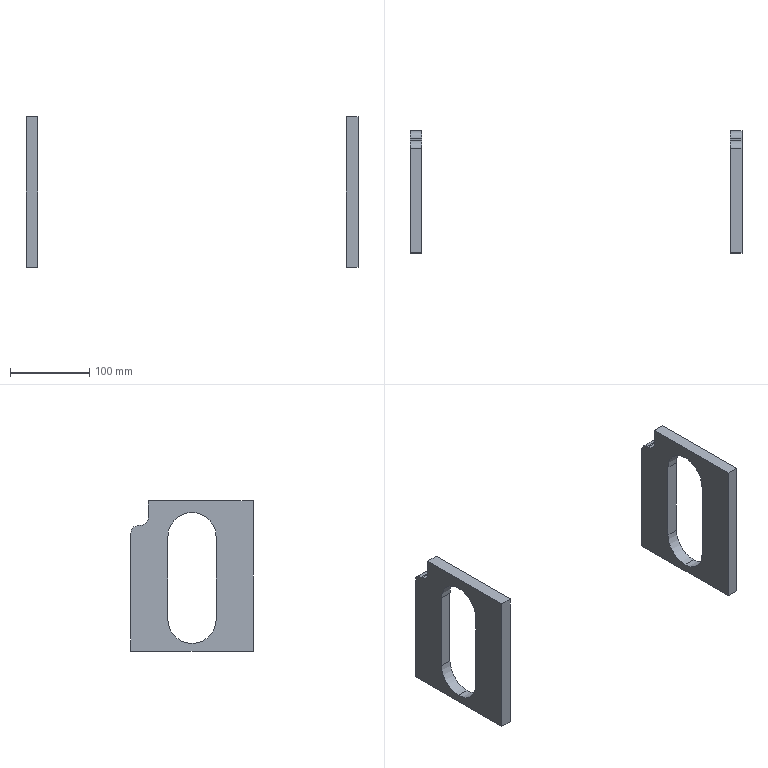Part | STEP file | Part 14^超升波生产线-2 | 2 solids | 30 faces | box 420 x 154.525 x 190 mm | volume 580946 mm3 | plane 20 | cylinder 10 | commonest cylinder face diameters 61.047 x6 20 x4
STEP:
#1=CARTESIAN_POINT('',(195.,0.,9.642));
#2=VERTEX_POINT('',#1);
#3=CARTESIAN_POINT('',(195.,30.523,40.165));
#4=VERTEX_POINT('',#3);
#5=CARTESIAN_POINT('',(195.,0.,40.165));
#6=DIRECTION('',(1.,0.,0.));
#7=DIRECTION('',(0.,1.,0.));
#8=AXIS2_PLACEMENT_3D('',#5,#6,#7);
#9=CIRCLE('',#8,30.523);
#10=EDGE_CURVE('',#2,#4,#9,.T.);
#11=ORIENTED_EDGE('',*,*,#10,.F.);
#12=CARTESIAN_POINT('',(210.,0.,9.642));
#13=VERTEX_POINT('',#12);
#14=CARTESIAN_POINT('',(-210.,0.,9.642));
#15=DIRECTION('',(1.,0.,0.));
#16=VECTOR('',#15,1000.);
#17=LINE('',#14,#16);
#18=EDGE_CURVE('',#2,#13,#17,.T.);
#19=ORIENTED_EDGE('',*,*,#18,.T.);
#20=CARTESIAN_POINT('',(210.,30.523,40.165));
#21=VERTEX_POINT('',#20);
#22=CARTESIAN_POINT('',(210.,0.,40.165));
#23=DIRECTION('',(1.,0.,0.));
#24=DIRECTION('',(0.,0.,-1.));
#25=AXIS2_PLACEMENT_3D('',#22,#23,#24);
#26=CIRCLE('',#25,30.523);
#27=EDGE_CURVE('',#13,#21,#26,.T.);
#28=ORIENTED_EDGE('',*,*,#27,.T.);
#29=CARTESIAN_POINT('',(-210.,30.523,40.165));
#30=DIRECTION('',(1.,0.,0.));
#31=VECTOR('',#30,1000.);
#32=LINE('',#29,#31);
#33=EDGE_CURVE('',#4,#21,#32,.T.);
#34=ORIENTED_EDGE('',*,*,#33,.F.);
#35=EDGE_LOOP('',(#11,#19,#28,#34));
#36=FACE_OUTER_BOUND('',#35,.T.);
#37=CARTESIAN_POINT('',(-210.,0.,40.165));
#38=DIRECTION('',(1.,0.,0.));
#39=DIRECTION('',(0.,0.,-1.));
#40=AXIS2_PLACEMENT_3D('',#37,#38,#39);
#41=CYLINDRICAL_SURFACE('',#40,30.523);
#42=ADVANCED_FACE('',(#36),#41,.F.);
#43=CARTESIAN_POINT('',(210.,-30.523,144.796));
#44=VERTEX_POINT('',#43);
#45=CARTESIAN_POINT('',(210.,-30.523,40.165));
#46=VERTEX_POINT('',#45);
#47=CARTESIAN_POINT('',(210.,-30.523,144.796));
#48=DIRECTION('',(0.,0.,-1.));
#49=VECTOR('',#48,1000.);
#50=LINE('',#47,#49);
#51=EDGE_CURVE('',#44,#46,#50,.T.);
#52=ORIENTED_EDGE('',*,*,#51,.F.);
#53=CARTESIAN_POINT('',(210.,30.523,144.796));
#54=VERTEX_POINT('',#53);
#55=CARTESIAN_POINT('',(210.,0.,144.796));
#56=DIRECTION('',(1.,0.,0.));
#57=DIRECTION('',(0.,0.,-1.));
#58=AXIS2_PLACEMENT_3D('',#55,#56,#57);
#59=CIRCLE('',#58,30.523);
#60=EDGE_CURVE('',#54,#44,#59,.T.);
#61=ORIENTED_EDGE('',*,*,#60,.F.);
#62=CARTESIAN_POINT('',(210.,30.523,144.796));
#63=DIRECTION('',(0.,0.,1.));
#64=VECTOR('',#63,1000.);
#65=LINE('',#62,#64);
#66=EDGE_CURVE('',#21,#54,#65,.T.);
#67=ORIENTED_EDGE('',*,*,#66,.F.);
#68=ORIENTED_EDGE('',*,*,#27,.F.);
#69=CARTESIAN_POINT('',(210.,0.,40.165));
#70=DIRECTION('',(1.,0.,0.));
#71=DIRECTION('',(0.,0.,-1.));
#72=AXIS2_PLACEMENT_3D('',#69,#70,#71);
#73=CIRCLE('',#72,30.523);
#74=EDGE_CURVE('',#46,#13,#73,.T.);
#75=ORIENTED_EDGE('',*,*,#74,.F.);
#76=EDGE_LOOP('',(#52,#61,#67,#68,#75));
#77=FACE_BOUND('',#76,.T.);
#78=CARTESIAN_POINT('',(210.,77.262,149.237));
#79=VERTEX_POINT('',#78);
#80=CARTESIAN_POINT('',(210.,77.262,0.));
#81=VERTEX_POINT('',#80);
#82=CARTESIAN_POINT('',(210.,77.262,190.));
#83=DIRECTION('',(0.,0.,-1.));
#84=VECTOR('',#83,1000.);
#85=LINE('',#82,#84);
#86=EDGE_CURVE('',#79,#81,#85,.T.);
#87=ORIENTED_EDGE('',*,*,#86,.F.);
#88=CARTESIAN_POINT('',(210.,67.262,159.237));
#89=VERTEX_POINT('',#88);
#90=CARTESIAN_POINT('',(210.,67.262,149.237));
#91=DIRECTION('',(1.,0.,0.));
#92=DIRECTION('',(0.,0.,1.));
#93=AXIS2_PLACEMENT_3D('',#90,#91,#92);
#94=CIRCLE('',#93,10.);
#95=EDGE_CURVE('',#79,#89,#94,.T.);
#96=ORIENTED_EDGE('',*,*,#95,.T.);
#97=CARTESIAN_POINT('',(210.,65.138,159.237));
#98=VERTEX_POINT('',#97);
#99=CARTESIAN_POINT('',(210.,79.238,159.237));
#100=DIRECTION('',(0.,-1.,0.));
#101=VECTOR('',#100,1000.);
#102=LINE('',#99,#101);
#103=EDGE_CURVE('',#89,#98,#102,.T.);
#104=ORIENTED_EDGE('',*,*,#103,.T.);
#105=CARTESIAN_POINT('',(210.,55.138,169.237));
#106=VERTEX_POINT('',#105);
#107=CARTESIAN_POINT('',(210.,65.138,169.237));
#108=DIRECTION('',(-1.,0.,0.));
#109=DIRECTION('',(0.,0.,1.));
#110=AXIS2_PLACEMENT_3D('',#107,#108,#109);
#111=CIRCLE('',#110,10.);
#112=EDGE_CURVE('',#98,#106,#111,.T.);
#113=ORIENTED_EDGE('',*,*,#112,.T.);
#114=CARTESIAN_POINT('',(210.,55.138,190.));
#115=VERTEX_POINT('',#114);
#116=CARTESIAN_POINT('',(210.,55.138,192.637));
#117=DIRECTION('',(0.,0.,1.));
#118=VECTOR('',#117,1000.);
#119=LINE('',#116,#118);
#120=EDGE_CURVE('',#106,#115,#119,.T.);
#121=ORIENTED_EDGE('',*,*,#120,.T.);
#122=CARTESIAN_POINT('',(210.,-77.262,190.));
#123=VERTEX_POINT('',#122);
#124=CARTESIAN_POINT('',(210.,77.262,190.));
#125=DIRECTION('',(0.,1.,0.));
#126=VECTOR('',#125,1000.);
#127=LINE('',#124,#126);
#128=EDGE_CURVE('',#123,#115,#127,.T.);
#129=ORIENTED_EDGE('',*,*,#128,.F.);
#130=CARTESIAN_POINT('',(210.,-77.262,0.));
#131=VERTEX_POINT('',#130);
#132=CARTESIAN_POINT('',(210.,-77.262,190.));
#133=DIRECTION('',(0.,0.,-1.));
#134=VECTOR('',#133,1000.);
#135=LINE('',#132,#134);
#136=EDGE_CURVE('',#123,#131,#135,.T.);
#137=ORIENTED_EDGE('',*,*,#136,.T.);
#138=CARTESIAN_POINT('',(210.,77.262,0.));
#139=DIRECTION('',(0.,1.,0.));
#140=VECTOR('',#139,1000.);
#141=LINE('',#138,#140);
#142=EDGE_CURVE('',#131,#81,#141,.T.);
#143=ORIENTED_EDGE('',*,*,#142,.T.);
#144=EDGE_LOOP('',(#87,#96,#104,#113,#121,#129,#137,#143));
#145=FACE_OUTER_BOUND('',#144,.T.);
#146=CARTESIAN_POINT('',(210.,77.262,190.));
#147=DIRECTION('',(-1.,0.,0.));
#148=DIRECTION('',(0.,0.,1.));
#149=AXIS2_PLACEMENT_3D('',#146,#147,#148);
#150=PLANE('',#149);
#151=ADVANCED_FACE('',(#77,#145),#150,.F.);
#152=CARTESIAN_POINT('',(195.,77.262,149.237));
#153=VERTEX_POINT('',#152);
#154=CARTESIAN_POINT('',(195.,77.262,0.));
#155=VERTEX_POINT('',#154);
#156=CARTESIAN_POINT('',(195.,77.262,190.));
#157=DIRECTION('',(0.,0.,-1.));
#158=VECTOR('',#157,1000.);
#159=LINE('',#156,#158);
#160=EDGE_CURVE('',#153,#155,#159,.T.);
#161=ORIENTED_EDGE('',*,*,#160,.F.);
#162=CARTESIAN_POINT('',(210.,77.262,149.237));
#163=DIRECTION('',(1.,0.,0.));
#164=VECTOR('',#163,1000.);
#165=LINE('',#162,#164);
#166=EDGE_CURVE('',#153,#79,#165,.T.);
#167=ORIENTED_EDGE('',*,*,#166,.T.);
#168=ORIENTED_EDGE('',*,*,#86,.T.);
#169=CARTESIAN_POINT('',(210.,77.262,0.));
#170=DIRECTION('',(-1.,0.,0.));
#171=VECTOR('',#170,1000.);
#172=LINE('',#169,#171);
#173=EDGE_CURVE('',#81,#155,#172,.T.);
#174=ORIENTED_EDGE('',*,*,#173,.T.);
#175=EDGE_LOOP('',(#161,#167,#168,#174));
#176=FACE_OUTER_BOUND('',#175,.T.);
#177=CARTESIAN_POINT('',(210.,77.262,190.));
#178=DIRECTION('',(0.,-1.,0.));
#179=DIRECTION('',(0.,0.,-1.));
#180=AXIS2_PLACEMENT_3D('',#177,#178,#179);
#181=PLANE('',#180);
#182=ADVANCED_FACE('',(#176),#181,.F.);
#183=CARTESIAN_POINT('',(195.,30.523,144.796));
#184=VERTEX_POINT('',#183);
#185=CARTESIAN_POINT('',(195.,30.523,190.));
#186=DIRECTION('',(0.,0.,1.));
#187=VECTOR('',#186,1000.);
#188=LINE('',#185,#187);
#189=EDGE_CURVE('',#4,#184,#188,.T.);
#190=ORIENTED_EDGE('',*,*,#189,.T.);
#191=CARTESIAN_POINT('',(195.,-30.523,144.796));
#192=VERTEX_POINT('',#191);
#193=CARTESIAN_POINT('',(195.,0.,144.796));
#194=DIRECTION('',(1.,0.,0.));
#195=DIRECTION('',(0.,1.,0.));
#196=AXIS2_PLACEMENT_3D('',#193,#194,#195);
#197=CIRCLE('',#196,30.523);
#198=EDGE_CURVE('',#184,#192,#197,.T.);
#199=ORIENTED_EDGE('',*,*,#198,.T.);
#200=CARTESIAN_POINT('',(195.,-30.523,40.165));
#201=VERTEX_POINT('',#200);
#202=CARTESIAN_POINT('',(195.,-30.523,190.));
#203=DIRECTION('',(0.,0.,-1.));
#204=VECTOR('',#203,1000.);
#205=LINE('',#202,#204);
#206=EDGE_CURVE('',#192,#201,#205,.T.);
#207=ORIENTED_EDGE('',*,*,#206,.T.);
#208=CARTESIAN_POINT('',(195.,0.,40.165));
#209=DIRECTION('',(1.,0.,0.));
#210=DIRECTION('',(0.,1.,0.));
#211=AXIS2_PLACEMENT_3D('',#208,#209,#210);
#212=CIRCLE('',#211,30.523);
#213=EDGE_CURVE('',#201,#2,#212,.T.);
#214=ORIENTED_EDGE('',*,*,#213,.T.);
#215=ORIENTED_EDGE('',*,*,#10,.T.);
#216=EDGE_LOOP('',(#190,#199,#207,#214,#215));
#217=FACE_BOUND('',#216,.T.);
#218=CARTESIAN_POINT('',(195.,65.138,159.237));
#219=VERTEX_POINT('',#218);
#220=CARTESIAN_POINT('',(195.,67.262,159.237));
#221=VERTEX_POINT('',#220);
#222=CARTESIAN_POINT('',(195.,77.262,159.237));
#223=DIRECTION('',(0.,1.,0.));
#224=VECTOR('',#223,1000.);
#225=LINE('',#222,#224);
#226=EDGE_CURVE('',#219,#221,#225,.T.);
#227=ORIENTED_EDGE('',*,*,#226,.T.);
#228=CARTESIAN_POINT('',(195.,67.262,149.237));
#229=DIRECTION('',(-1.,0.,0.));
#230=DIRECTION('',(0.,1.,0.));
#231=AXIS2_PLACEMENT_3D('',#228,#229,#230);
#232=CIRCLE('',#231,10.);
#233=EDGE_CURVE('',#221,#153,#232,.T.);
#234=ORIENTED_EDGE('',*,*,#233,.T.);
#235=ORIENTED_EDGE('',*,*,#160,.T.);
#236=CARTESIAN_POINT('',(195.,-77.262,0.));
#237=VERTEX_POINT('',#236);
#238=CARTESIAN_POINT('',(195.,77.262,0.));
#239=DIRECTION('',(0.,-1.,0.));
#240=VECTOR('',#239,1000.);
#241=LINE('',#238,#240);
#242=EDGE_CURVE('',#155,#237,#241,.T.);
#243=ORIENTED_EDGE('',*,*,#242,.T.);
#244=CARTESIAN_POINT('',(195.,-77.262,190.));
#245=VERTEX_POINT('',#244);
#246=CARTESIAN_POINT('',(195.,-77.262,190.));
#247=DIRECTION('',(0.,0.,-1.));
#248=VECTOR('',#247,1000.);
#249=LINE('',#246,#248);
#250=EDGE_CURVE('',#245,#237,#249,.T.);
#251=ORIENTED_EDGE('',*,*,#250,.F.);
#252=CARTESIAN_POINT('',(195.,55.138,190.));
#253=VERTEX_POINT('',#252);
#254=CARTESIAN_POINT('',(195.,77.262,190.));
#255=DIRECTION('',(0.,-1.,0.));
#256=VECTOR('',#255,1000.);
#257=LINE('',#254,#256);
#258=EDGE_CURVE('',#253,#245,#257,.T.);
#259=ORIENTED_EDGE('',*,*,#258,.F.);
#260=CARTESIAN_POINT('',(195.,55.138,169.237));
#261=VERTEX_POINT('',#260);
#262=CARTESIAN_POINT('',(195.,55.138,190.));
#263=DIRECTION('',(0.,0.,-1.));
#264=VECTOR('',#263,1000.);
#265=LINE('',#262,#264);
#266=EDGE_CURVE('',#253,#261,#265,.T.);
#267=ORIENTED_EDGE('',*,*,#266,.T.);
#268=CARTESIAN_POINT('',(195.,65.138,169.237));
#269=DIRECTION('',(1.,0.,0.));
#270=DIRECTION('',(0.,1.,0.));
#271=AXIS2_PLACEMENT_3D('',#268,#269,#270);
#272=CIRCLE('',#271,10.);
#273=EDGE_CURVE('',#261,#219,#272,.T.);
#274=ORIENTED_EDGE('',*,*,#273,.T.);
#275=EDGE_LOOP('',(#227,#234,#235,#243,#251,#259,#267,#274));
#276=FACE_OUTER_BOUND('',#275,.T.);
#277=CARTESIAN_POINT('',(195.,77.262,190.));
#278=DIRECTION('',(1.,0.,0.));
#279=DIRECTION('',(0.,1.,0.));
#280=AXIS2_PLACEMENT_3D('',#277,#278,#279);
#281=PLANE('',#280);
#282=ADVANCED_FACE('',(#217,#276),#281,.F.);
#283=CARTESIAN_POINT('',(210.,-77.262,0.));
#284=DIRECTION('',(1.,0.,0.));
#285=VECTOR('',#284,1000.);
#286=LINE('',#283,#285);
#287=EDGE_CURVE('',#237,#131,#286,.T.);
#288=ORIENTED_EDGE('',*,*,#287,.T.);
#289=ORIENTED_EDGE('',*,*,#136,.F.);
#290=CARTESIAN_POINT('',(210.,-77.262,190.));
#291=DIRECTION('',(1.,0.,0.));
#292=VECTOR('',#291,1000.);
#293=LINE('',#290,#292);
#294=EDGE_CURVE('',#245,#123,#293,.T.);
#295=ORIENTED_EDGE('',*,*,#294,.F.);
#296=ORIENTED_EDGE('',*,*,#250,.T.);
#297=EDGE_LOOP('',(#288,#289,#295,#296));
#298=FACE_OUTER_BOUND('',#297,.T.);
#299=CARTESIAN_POINT('',(210.,-77.262,190.));
#300=DIRECTION('',(0.,1.,0.));
#301=DIRECTION('',(0.,0.,1.));
#302=AXIS2_PLACEMENT_3D('',#299,#300,#301);
#303=PLANE('',#302);
#304=ADVANCED_FACE('',(#298),#303,.F.);
#305=ORIENTED_EDGE('',*,*,#128,.T.);
#306=CARTESIAN_POINT('',(210.,55.138,190.));
#307=DIRECTION('',(-1.,0.,0.));
#308=VECTOR('',#307,1000.);
#309=LINE('',#306,#308);
#310=EDGE_CURVE('',#115,#253,#309,.T.);
#311=ORIENTED_EDGE('',*,*,#310,.T.);
#312=ORIENTED_EDGE('',*,*,#258,.T.);
#313=ORIENTED_EDGE('',*,*,#294,.T.);
#314=EDGE_LOOP('',(#305,#311,#312,#313));
#315=FACE_OUTER_BOUND('',#314,.T.);
#316=CARTESIAN_POINT('',(210.,-77.262,190.));
#317=DIRECTION('',(0.,0.,-1.));
#318=DIRECTION('',(-1.,0.,0.));
#319=AXIS2_PLACEMENT_3D('',#316,#317,#318);
#320=PLANE('',#319);
#321=ADVANCED_FACE('',(#315),#320,.F.);
#322=ORIENTED_EDGE('',*,*,#142,.F.);
#323=ORIENTED_EDGE('',*,*,#287,.F.);
#324=ORIENTED_EDGE('',*,*,#242,.F.);
#325=ORIENTED_EDGE('',*,*,#173,.F.);
#326=EDGE_LOOP('',(#322,#323,#324,#325));
#327=FACE_OUTER_BOUND('',#326,.T.);
#328=CARTESIAN_POINT('',(210.,-77.262,0.));
#329=DIRECTION('',(0.,0.,-1.));
#330=DIRECTION('',(-1.,0.,0.));
#331=AXIS2_PLACEMENT_3D('',#328,#329,#330);
#332=PLANE('',#331);
#333=ADVANCED_FACE('',(#327),#332,.T.);
#334=CARTESIAN_POINT('',(-210.,30.523,144.796));
#335=DIRECTION('',(1.,0.,0.));
#336=VECTOR('',#335,1000.);
#337=LINE('',#334,#336);
#338=EDGE_CURVE('',#184,#54,#337,.T.);
#339=ORIENTED_EDGE('',*,*,#338,.T.);
#340=ORIENTED_EDGE('',*,*,#60,.T.);
#341=CARTESIAN_POINT('',(-210.,-30.523,144.796));
#342=DIRECTION('',(1.,0.,0.));
#343=VECTOR('',#342,1000.);
#344=LINE('',#341,#343);
#345=EDGE_CURVE('',#192,#44,#344,.T.);
#346=ORIENTED_EDGE('',*,*,#345,.F.);
#347=ORIENTED_EDGE('',*,*,#198,.F.);
#348=EDGE_LOOP('',(#339,#340,#346,#347));
#349=FACE_OUTER_BOUND('',#348,.T.);
#350=CARTESIAN_POINT('',(-210.,0.,144.796));
#351=DIRECTION('',(1.,0.,0.));
#352=DIRECTION('',(0.,0.,-1.));
#353=AXIS2_PLACEMENT_3D('',#350,#351,#352);
#354=CYLINDRICAL_SURFACE('',#353,30.523);
#355=ADVANCED_FACE('',(#349),#354,.F.);
#356=ORIENTED_EDGE('',*,*,#33,.T.);
#357=ORIENTED_EDGE('',*,*,#66,.T.);
#358=ORIENTED_EDGE('',*,*,#338,.F.);
#359=ORIENTED_EDGE('',*,*,#189,.F.);
#360=EDGE_LOOP('',(#356,#357,#358,#359));
#361=FACE_OUTER_BOUND('',#360,.T.);
#362=CARTESIAN_POINT('',(-210.,30.523,144.796));
#363=DIRECTION('',(0.,1.,0.));
#364=DIRECTION('',(0.,0.,1.));
#365=AXIS2_PLACEMENT_3D('',#362,#363,#364);
#366=PLANE('',#365);
#367=ADVANCED_FACE('',(#361),#366,.F.);
#368=ORIENTED_EDGE('',*,*,#18,.F.);
#369=ORIENTED_EDGE('',*,*,#213,.F.);
#370=CARTESIAN_POINT('',(-210.,-30.523,40.165));
#371=DIRECTION('',(1.,0.,0.));
#372=VECTOR('',#371,1000.);
#373=LINE('',#370,#372);
#374=EDGE_CURVE('',#201,#46,#373,.T.);
#375=ORIENTED_EDGE('',*,*,#374,.T.);
#376=ORIENTED_EDGE('',*,*,#74,.T.);
#377=EDGE_LOOP('',(#368,#369,#375,#376));
#378=FACE_OUTER_BOUND('',#377,.T.);
#379=CARTESIAN_POINT('',(-210.,0.,40.165));
#380=DIRECTION('',(1.,0.,0.));
#381=DIRECTION('',(0.,0.,-1.));
#382=AXIS2_PLACEMENT_3D('',#379,#380,#381);
#383=CYLINDRICAL_SURFACE('',#382,30.523);
#384=ADVANCED_FACE('',(#378),#383,.F.);
#385=ORIENTED_EDGE('',*,*,#345,.T.);
#386=ORIENTED_EDGE('',*,*,#51,.T.);
#387=ORIENTED_EDGE('',*,*,#374,.F.);
#388=ORIENTED_EDGE('',*,*,#206,.F.);
#389=EDGE_LOOP('',(#385,#386,#387,#388));
#390=FACE_OUTER_BOUND('',#389,.T.);
#391=CARTESIAN_POINT('',(-210.,-30.523,144.796));
#392=DIRECTION('',(0.,-1.,0.));
#393=DIRECTION('',(0.,0.,-1.));
#394=AXIS2_PLACEMENT_3D('',#391,#392,#393);
#395=PLANE('',#394);
#396=ADVANCED_FACE('',(#390),#395,.F.);
#397=ORIENTED_EDGE('',*,*,#103,.F.);
#398=CARTESIAN_POINT('',(210.,67.262,159.237));
#399=DIRECTION('',(-1.,0.,0.));
#400=VECTOR('',#399,1000.);
#401=LINE('',#398,#400);
#402=EDGE_CURVE('',#89,#221,#401,.T.);
#403=ORIENTED_EDGE('',*,*,#402,.T.);
#404=ORIENTED_EDGE('',*,*,#226,.F.);
#405=CARTESIAN_POINT('',(210.,65.138,159.237));
#406=DIRECTION('',(1.,0.,0.));
#407=VECTOR('',#406,1000.);
#408=LINE('',#405,#407);
#409=EDGE_CURVE('',#219,#98,#408,.T.);
#410=ORIENTED_EDGE('',*,*,#409,.T.);
#411=EDGE_LOOP('',(#397,#403,#404,#410));
#412=FACE_OUTER_BOUND('',#411,.T.);
#413=CARTESIAN_POINT('',(210.,79.238,159.237));
#414=DIRECTION('',(0.,0.,-1.));
#415=DIRECTION('',(-1.,0.,0.));
#416=AXIS2_PLACEMENT_3D('',#413,#414,#415);
#417=PLANE('',#416);
#418=ADVANCED_FACE('',(#412),#417,.F.);
#419=ORIENTED_EDGE('',*,*,#120,.F.);
#420=CARTESIAN_POINT('',(195.,55.138,169.237));
#421=DIRECTION('',(-1.,0.,0.));
#422=VECTOR('',#421,1000.);
#423=LINE('',#420,#422);
#424=EDGE_CURVE('',#106,#261,#423,.T.);
#425=ORIENTED_EDGE('',*,*,#424,.T.);
#426=ORIENTED_EDGE('',*,*,#266,.F.);
#427=ORIENTED_EDGE('',*,*,#310,.F.);
#428=EDGE_LOOP('',(#419,#425,#426,#427));
#429=FACE_OUTER_BOUND('',#428,.T.);
#430=CARTESIAN_POINT('',(210.,55.138,192.637));
#431=DIRECTION('',(0.,-1.,0.));
#432=DIRECTION('',(0.,0.,-1.));
#433=AXIS2_PLACEMENT_3D('',#430,#431,#432);
#434=PLANE('',#433);
#435=ADVANCED_FACE('',(#429),#434,.F.);
#436=ORIENTED_EDGE('',*,*,#233,.F.);
#437=ORIENTED_EDGE('',*,*,#402,.F.);
#438=ORIENTED_EDGE('',*,*,#95,.F.);
#439=ORIENTED_EDGE('',*,*,#166,.F.);
#440=EDGE_LOOP('',(#436,#437,#438,#439));
#441=FACE_OUTER_BOUND('',#440,.T.);
#442=CARTESIAN_POINT('',(210.,67.262,149.237));
#443=DIRECTION('',(1.,0.,0.));
#444=DIRECTION('',(0.,0.,-1.));
#445=AXIS2_PLACEMENT_3D('',#442,#443,#444);
#446=CYLINDRICAL_SURFACE('',#445,10.);
#447=ADVANCED_FACE('',(#441),#446,.T.);
#448=ORIENTED_EDGE('',*,*,#112,.F.);
#449=ORIENTED_EDGE('',*,*,#409,.F.);
#450=ORIENTED_EDGE('',*,*,#273,.F.);
#451=ORIENTED_EDGE('',*,*,#424,.F.);
#452=EDGE_LOOP('',(#448,#449,#450,#451));
#453=FACE_OUTER_BOUND('',#452,.T.);
#454=CARTESIAN_POINT('',(210.,65.138,169.237));
#455=DIRECTION('',(1.,0.,0.));
#456=DIRECTION('',(0.,0.,-1.));
#457=AXIS2_PLACEMENT_3D('',#454,#455,#456);
#458=CYLINDRICAL_SURFACE('',#457,10.);
#459=ADVANCED_FACE('',(#453),#458,.F.);
#460=CLOSED_SHELL('',(#42,#151,#182,#282,#304,#321,#333,#355,#367,#384,#396,#418,#435,#447,#459));
#461=MANIFOLD_SOLID_BREP('',#460);
#462=CARTESIAN_POINT('',(-210.,0.,9.642));
#463=VERTEX_POINT('',#462);
#464=CARTESIAN_POINT('',(-210.,30.523,40.165));
#465=VERTEX_POINT('',#464);
#466=CARTESIAN_POINT('',(-210.,0.,40.165));
#467=DIRECTION('',(1.,0.,0.));
#468=DIRECTION('',(0.,0.,-1.));
#469=AXIS2_PLACEMENT_3D('',#466,#467,#468);
#470=CIRCLE('',#469,30.523);
#471=EDGE_CURVE('',#463,#465,#470,.T.);
#472=ORIENTED_EDGE('',*,*,#471,.F.);
#473=CARTESIAN_POINT('',(-195.,0.,9.642));
#474=VERTEX_POINT('',#473);
#475=CARTESIAN_POINT('',(-210.,0.,9.642));
#476=DIRECTION('',(1.,0.,0.));
#477=VECTOR('',#476,1000.);
#478=LINE('',#475,#477);
#479=EDGE_CURVE('',#463,#474,#478,.T.);
#480=ORIENTED_EDGE('',*,*,#479,.T.);
#481=CARTESIAN_POINT('',(-195.,30.523,40.165));
#482=VERTEX_POINT('',#481);
#483=CARTESIAN_POINT('',(-195.,0.,40.165));
#484=DIRECTION('',(-1.,0.,0.));
#485=DIRECTION('',(0.,-1.,0.));
#486=AXIS2_PLACEMENT_3D('',#483,#484,#485);
#487=CIRCLE('',#486,30.523);
#488=EDGE_CURVE('',#482,#474,#487,.T.);
#489=ORIENTED_EDGE('',*,*,#488,.F.);
#490=CARTESIAN_POINT('',(-210.,30.523,40.165));
#491=DIRECTION('',(1.,0.,0.));
#492=VECTOR('',#491,1000.);
#493=LINE('',#490,#492);
#494=EDGE_CURVE('',#465,#482,#493,.T.);
#495=ORIENTED_EDGE('',*,*,#494,.F.);
#496=EDGE_LOOP('',(#472,#480,#489,#495));
#497=FACE_OUTER_BOUND('',#496,.T.);
#498=CARTESIAN_POINT('',(-210.,0.,40.165));
#499=DIRECTION('',(1.,0.,0.));
#500=DIRECTION('',(0.,0.,-1.));
#501=AXIS2_PLACEMENT_3D('',#498,#499,#500);
#502=CYLINDRICAL_SURFACE('',#501,30.523);
#503=ADVANCED_FACE('',(#497),#502,.F.);
#504=CARTESIAN_POINT('',(-210.,30.523,144.796));
#505=VERTEX_POINT('',#504);
#506=CARTESIAN_POINT('',(-210.,30.523,144.796));
#507=DIRECTION('',(0.,0.,1.));
#508=VECTOR('',#507,1000.);
#509=LINE('',#506,#508);
#510=EDGE_CURVE('',#465,#505,#509,.T.);
#511=ORIENTED_EDGE('',*,*,#510,.T.);
#512=CARTESIAN_POINT('',(-210.,-30.523,144.796));
#513=VERTEX_POINT('',#512);
#514=CARTESIAN_POINT('',(-210.,0.,144.796));
#515=DIRECTION('',(1.,0.,0.));
#516=DIRECTION('',(0.,0.,-1.));
#517=AXIS2_PLACEMENT_3D('',#514,#515,#516);
#518=CIRCLE('',#517,30.523);
#519=EDGE_CURVE('',#505,#513,#518,.T.);
#520=ORIENTED_EDGE('',*,*,#519,.T.);
#521=CARTESIAN_POINT('',(-210.,-30.523,40.165));
#522=VERTEX_POINT('',#521);
#523=CARTESIAN_POINT('',(-210.,-30.523,144.796));
#524=DIRECTION('',(0.,0.,-1.));
#525=VECTOR('',#524,1000.);
#526=LINE('',#523,#525);
#527=EDGE_CURVE('',#513,#522,#526,.T.);
#528=ORIENTED_EDGE('',*,*,#527,.T.);
#529=CARTESIAN_POINT('',(-210.,0.,40.165));
#530=DIRECTION('',(1.,0.,0.));
#531=DIRECTION('',(0.,0.,-1.));
#532=AXIS2_PLACEMENT_3D('',#529,#530,#531);
#533=CIRCLE('',#532,30.523);
#534=EDGE_CURVE('',#522,#463,#533,.T.);
#535=ORIENTED_EDGE('',*,*,#534,.T.);
#536=ORIENTED_EDGE('',*,*,#471,.T.);
#537=EDGE_LOOP('',(#511,#520,#528,#535,#536));
#538=FACE_BOUND('',#537,.T.);
#539=CARTESIAN_POINT('',(-210.,67.262,159.237));
#540=VERTEX_POINT('',#539);
#541=CARTESIAN_POINT('',(-210.,65.138,159.237));
#542=VERTEX_POINT('',#541);
#543=CARTESIAN_POINT('',(-210.,79.238,159.237));
#544=DIRECTION('',(0.,-1.,0.));
#545=VECTOR('',#544,1000.);
#546=LINE('',#543,#545);
#547=EDGE_CURVE('',#540,#542,#546,.T.);
#548=ORIENTED_EDGE('',*,*,#547,.F.);
#549=CARTESIAN_POINT('',(-210.,77.262,149.237));
#550=VERTEX_POINT('',#549);
#551=CARTESIAN_POINT('',(-210.,67.262,149.237));
#552=DIRECTION('',(-1.,0.,0.));
#553=DIRECTION('',(0.,0.,-1.));
#554=AXIS2_PLACEMENT_3D('',#551,#552,#553);
#555=CIRCLE('',#554,10.);
#556=EDGE_CURVE('',#540,#550,#555,.T.);
#557=ORIENTED_EDGE('',*,*,#556,.T.);
#558=CARTESIAN_POINT('',(-210.,77.262,0.));
#559=VERTEX_POINT('',#558);
#560=CARTESIAN_POINT('',(-210.,77.262,190.));
#561=DIRECTION('',(0.,0.,-1.));
#562=VECTOR('',#561,1000.);
#563=LINE('',#560,#562);
#564=EDGE_CURVE('',#550,#559,#563,.T.);
#565=ORIENTED_EDGE('',*,*,#564,.T.);
#566=CARTESIAN_POINT('',(-210.,-77.262,0.));
#567=VERTEX_POINT('',#566);
#568=CARTESIAN_POINT('',(-210.,77.262,0.));
#569=DIRECTION('',(0.,-1.,0.));
#570=VECTOR('',#569,1000.);
#571=LINE('',#568,#570);
#572=EDGE_CURVE('',#559,#567,#571,.T.);
#573=ORIENTED_EDGE('',*,*,#572,.T.);
#574=CARTESIAN_POINT('',(-210.,-77.262,190.));
#575=VERTEX_POINT('',#574);
#576=CARTESIAN_POINT('',(-210.,-77.262,190.));
#577=DIRECTION('',(0.,0.,-1.));
#578=VECTOR('',#577,1000.);
#579=LINE('',#576,#578);
#580=EDGE_CURVE('',#575,#567,#579,.T.);
#581=ORIENTED_EDGE('',*,*,#580,.F.);
#582=CARTESIAN_POINT('',(-210.,55.138,190.));
#583=VERTEX_POINT('',#582);
#584=CARTESIAN_POINT('',(-210.,77.262,190.));
#585=DIRECTION('',(0.,-1.,0.));
#586=VECTOR('',#585,1000.);
#587=LINE('',#584,#586);
#588=EDGE_CURVE('',#583,#575,#587,.T.);
#589=ORIENTED_EDGE('',*,*,#588,.F.);
#590=CARTESIAN_POINT('',(-210.,55.138,169.237));
#591=VERTEX_POINT('',#590);
#592=CARTESIAN_POINT('',(-210.,55.138,192.637));
#593=DIRECTION('',(0.,0.,1.));
#594=VECTOR('',#593,1000.);
#595=LINE('',#592,#594);
#596=EDGE_CURVE('',#591,#583,#595,.T.);
#597=ORIENTED_EDGE('',*,*,#596,.F.);
#598=CARTESIAN_POINT('',(-210.,65.138,169.237));
#599=DIRECTION('',(1.,0.,0.));
#600=DIRECTION('',(0.,0.,-1.));
#601=AXIS2_PLACEMENT_3D('',#598,#599,#600);
#602=CIRCLE('',#601,10.);
#603=EDGE_CURVE('',#591,#542,#602,.T.);
#604=ORIENTED_EDGE('',*,*,#603,.T.);
#605=EDGE_LOOP('',(#548,#557,#565,#573,#581,#589,#597,#604));
#606=FACE_OUTER_BOUND('',#605,.T.);
#607=CARTESIAN_POINT('',(-210.,77.262,190.));
#608=DIRECTION('',(1.,0.,0.));
#609=DIRECTION('',(0.,0.,-1.));
#610=AXIS2_PLACEMENT_3D('',#607,#608,#609);
#611=PLANE('',#610);
#612=ADVANCED_FACE('',(#538,#606),#611,.F.);
#613=CARTESIAN_POINT('',(-195.,-77.262,0.));
#614=VERTEX_POINT('',#613);
#615=CARTESIAN_POINT('',(-210.,-77.262,0.));
#616=DIRECTION('',(1.,0.,0.));
#617=VECTOR('',#616,1000.);
#618=LINE('',#615,#617);
#619=EDGE_CURVE('',#567,#614,#618,.T.);
#620=ORIENTED_EDGE('',*,*,#619,.T.);
#621=CARTESIAN_POINT('',(-195.,-77.262,190.));
#622=VERTEX_POINT('',#621);
#623=CARTESIAN_POINT('',(-195.,-77.262,190.));
#624=DIRECTION('',(0.,0.,-1.));
#625=VECTOR('',#624,1000.);
#626=LINE('',#623,#625);
#627=EDGE_CURVE('',#622,#614,#626,.T.);
#628=ORIENTED_EDGE('',*,*,#627,.F.);
#629=CARTESIAN_POINT('',(-210.,-77.262,190.));
#630=DIRECTION('',(1.,0.,0.));
#631=VECTOR('',#630,1000.);
#632=LINE('',#629,#631);
#633=EDGE_CURVE('',#575,#622,#632,.T.);
#634=ORIENTED_EDGE('',*,*,#633,.F.);
#635=ORIENTED_EDGE('',*,*,#580,.T.);
#636=EDGE_LOOP('',(#620,#628,#634,#635));
#637=FACE_OUTER_BOUND('',#636,.T.);
#638=CARTESIAN_POINT('',(-210.,-77.262,190.));
#639=DIRECTION('',(0.,1.,0.));
#640=DIRECTION('',(0.,0.,1.));
#641=AXIS2_PLACEMENT_3D('',#638,#639,#640);
#642=PLANE('',#641);
#643=ADVANCED_FACE('',(#637),#642,.F.);
#644=CARTESIAN_POINT('',(-195.,-30.523,40.165));
#645=VERTEX_POINT('',#644);
#646=CARTESIAN_POINT('',(-195.,-30.523,144.796));
#647=VERTEX_POINT('',#646);
#648=CARTESIAN_POINT('',(-195.,-30.523,190.));
#649=DIRECTION('',(0.,0.,1.));
#650=VECTOR('',#649,1000.);
#651=LINE('',#648,#650);
#652=EDGE_CURVE('',#645,#647,#651,.T.);
#653=ORIENTED_EDGE('',*,*,#652,.T.);
#654=CARTESIAN_POINT('',(-195.,30.523,144.796));
#655=VERTEX_POINT('',#654);
#656=CARTESIAN_POINT('',(-195.,0.,144.796));
#657=DIRECTION('',(-1.,0.,0.));
#658=DIRECTION('',(0.,-1.,0.));
#659=AXIS2_PLACEMENT_3D('',#656,#657,#658);
#660=CIRCLE('',#659,30.523);
#661=EDGE_CURVE('',#647,#655,#660,.T.);
#662=ORIENTED_EDGE('',*,*,#661,.T.);
#663=CARTESIAN_POINT('',(-195.,30.523,190.));
#664=DIRECTION('',(0.,0.,-1.));
#665=VECTOR('',#664,1000.);
#666=LINE('',#663,#665);
#667=EDGE_CURVE('',#655,#482,#666,.T.);
#668=ORIENTED_EDGE('',*,*,#667,.T.);
#669=ORIENTED_EDGE('',*,*,#488,.T.);
#670=CARTESIAN_POINT('',(-195.,0.,40.165));
#671=DIRECTION('',(-1.,0.,0.));
#672=DIRECTION('',(0.,-1.,0.));
#673=AXIS2_PLACEMENT_3D('',#670,#671,#672);
#674=CIRCLE('',#673,30.523);
#675=EDGE_CURVE('',#474,#645,#674,.T.);
#676=ORIENTED_EDGE('',*,*,#675,.T.);
#677=EDGE_LOOP('',(#653,#662,#668,#669,#676));
#678=FACE_BOUND('',#677,.T.);
#679=CARTESIAN_POINT('',(-195.,77.262,149.237));
#680=VERTEX_POINT('',#679);
#681=CARTESIAN_POINT('',(-195.,77.262,0.));
#682=VERTEX_POINT('',#681);
#683=CARTESIAN_POINT('',(-195.,77.262,190.));
#684=DIRECTION('',(0.,0.,-1.));
#685=VECTOR('',#684,1000.);
#686=LINE('',#683,#685);
#687=EDGE_CURVE('',#680,#682,#686,.T.);
#688=ORIENTED_EDGE('',*,*,#687,.F.);
#689=CARTESIAN_POINT('',(-195.,67.262,159.237));
#690=VERTEX_POINT('',#689);
#691=CARTESIAN_POINT('',(-195.,67.262,149.237));
#692=DIRECTION('',(1.,0.,0.));
#693=DIRECTION('',(0.,-1.,0.));
#694=AXIS2_PLACEMENT_3D('',#691,#692,#693);
#695=CIRCLE('',#694,10.);
#696=EDGE_CURVE('',#680,#690,#695,.T.);
#697=ORIENTED_EDGE('',*,*,#696,.T.);
#698=CARTESIAN_POINT('',(-195.,65.138,159.237));
#699=VERTEX_POINT('',#698);
#700=CARTESIAN_POINT('',(-195.,77.262,159.237));
#701=DIRECTION('',(0.,-1.,0.));
#702=VECTOR('',#701,1000.);
#703=LINE('',#700,#702);
#704=EDGE_CURVE('',#690,#699,#703,.T.);
#705=ORIENTED_EDGE('',*,*,#704,.T.);
#706=CARTESIAN_POINT('',(-195.,55.138,169.237));
#707=VERTEX_POINT('',#706);
#708=CARTESIAN_POINT('',(-195.,65.138,169.237));
#709=DIRECTION('',(-1.,0.,0.));
#710=DIRECTION('',(0.,-1.,0.));
#711=AXIS2_PLACEMENT_3D('',#708,#709,#710);
#712=CIRCLE('',#711,10.);
#713=EDGE_CURVE('',#699,#707,#712,.T.);
#714=ORIENTED_EDGE('',*,*,#713,.T.);
#715=CARTESIAN_POINT('',(-195.,55.138,190.));
#716=VERTEX_POINT('',#715);
#717=CARTESIAN_POINT('',(-195.,55.138,190.));
#718=DIRECTION('',(0.,0.,1.));
#719=VECTOR('',#718,1000.);
#720=LINE('',#717,#719);
#721=EDGE_CURVE('',#707,#716,#720,.T.);
#722=ORIENTED_EDGE('',*,*,#721,.T.);
#723=CARTESIAN_POINT('',(-195.,77.262,190.));
#724=DIRECTION('',(0.,1.,0.));
#725=VECTOR('',#724,1000.);
#726=LINE('',#723,#725);
#727=EDGE_CURVE('',#622,#716,#726,.T.);
#728=ORIENTED_EDGE('',*,*,#727,.F.);
#729=ORIENTED_EDGE('',*,*,#627,.T.);
#730=CARTESIAN_POINT('',(-195.,77.262,0.));
#731=DIRECTION('',(0.,1.,0.));
#732=VECTOR('',#731,1000.);
#733=LINE('',#730,#732);
#734=EDGE_CURVE('',#614,#682,#733,.T.);
#735=ORIENTED_EDGE('',*,*,#734,.T.);
#736=EDGE_LOOP('',(#688,#697,#705,#714,#722,#728,#729,#735));
#737=FACE_OUTER_BOUND('',#736,.T.);
#738=CARTESIAN_POINT('',(-195.,77.262,190.));
#739=DIRECTION('',(-1.,0.,0.));
#740=DIRECTION('',(0.,-1.,0.));
#741=AXIS2_PLACEMENT_3D('',#738,#739,#740);
#742=PLANE('',#741);
#743=ADVANCED_FACE('',(#678,#737),#742,.F.);
#744=ORIENTED_EDGE('',*,*,#564,.F.);
#745=CARTESIAN_POINT('',(-210.,77.262,149.237));
#746=DIRECTION('',(1.,0.,0.));
#747=VECTOR('',#746,1000.);
#748=LINE('',#745,#747);
#749=EDGE_CURVE('',#550,#680,#748,.T.);
#750=ORIENTED_EDGE('',*,*,#749,.T.);
#751=ORIENTED_EDGE('',*,*,#687,.T.);
#752=CARTESIAN_POINT('',(-210.,77.262,0.));
#753=DIRECTION('',(-1.,0.,0.));
#754=VECTOR('',#753,1000.);
#755=LINE('',#752,#754);
#756=EDGE_CURVE('',#682,#559,#755,.T.);
#757=ORIENTED_EDGE('',*,*,#756,.T.);
#758=EDGE_LOOP('',(#744,#750,#751,#757));
#759=FACE_OUTER_BOUND('',#758,.T.);
#760=CARTESIAN_POINT('',(-210.,77.262,190.));
#761=DIRECTION('',(0.,-1.,0.));
#762=DIRECTION('',(0.,0.,-1.));
#763=AXIS2_PLACEMENT_3D('',#760,#761,#762);
#764=PLANE('',#763);
#765=ADVANCED_FACE('',(#759),#764,.F.);
#766=CARTESIAN_POINT('',(-210.,55.138,190.));
#767=DIRECTION('',(1.,0.,0.));
#768=VECTOR('',#767,1000.);
#769=LINE('',#766,#768);
#770=EDGE_CURVE('',#583,#716,#769,.T.);
#771=ORIENTED_EDGE('',*,*,#770,.F.);
#772=ORIENTED_EDGE('',*,*,#588,.T.);
#773=ORIENTED_EDGE('',*,*,#633,.T.);
#774=ORIENTED_EDGE('',*,*,#727,.T.);
#775=EDGE_LOOP('',(#771,#772,#773,#774));
#776=FACE_OUTER_BOUND('',#775,.T.);
#777=CARTESIAN_POINT('',(-210.,-77.262,190.));
#778=DIRECTION('',(0.,0.,1.));
#779=DIRECTION('',(1.,0.,0.));
#780=AXIS2_PLACEMENT_3D('',#777,#778,#779);
#781=PLANE('',#780);
#782=ADVANCED_FACE('',(#776),#781,.T.);
#783=ORIENTED_EDGE('',*,*,#572,.F.);
#784=ORIENTED_EDGE('',*,*,#756,.F.);
#785=ORIENTED_EDGE('',*,*,#734,.F.);
#786=ORIENTED_EDGE('',*,*,#619,.F.);
#787=EDGE_LOOP('',(#783,#784,#785,#786));
#788=FACE_OUTER_BOUND('',#787,.T.);
#789=CARTESIAN_POINT('',(-210.,-77.262,0.));
#790=DIRECTION('',(0.,0.,1.));
#791=DIRECTION('',(1.,0.,0.));
#792=AXIS2_PLACEMENT_3D('',#789,#790,#791);
#793=PLANE('',#792);
#794=ADVANCED_FACE('',(#788),#793,.F.);
#795=CARTESIAN_POINT('',(-210.,-30.523,144.796));
#796=DIRECTION('',(1.,0.,0.));
#797=VECTOR('',#796,1000.);
#798=LINE('',#795,#797);
#799=EDGE_CURVE('',#513,#647,#798,.T.);
#800=ORIENTED_EDGE('',*,*,#799,.F.);
#801=ORIENTED_EDGE('',*,*,#519,.F.);
#802=CARTESIAN_POINT('',(-210.,30.523,144.796));
#803=DIRECTION('',(1.,0.,0.));
#804=VECTOR('',#803,1000.);
#805=LINE('',#802,#804);
#806=EDGE_CURVE('',#505,#655,#805,.T.);
#807=ORIENTED_EDGE('',*,*,#806,.T.);
#808=ORIENTED_EDGE('',*,*,#661,.F.);
#809=EDGE_LOOP('',(#800,#801,#807,#808));
#810=FACE_OUTER_BOUND('',#809,.T.);
#811=CARTESIAN_POINT('',(-210.,0.,144.796));
#812=DIRECTION('',(1.,0.,0.));
#813=DIRECTION('',(0.,0.,-1.));
#814=AXIS2_PLACEMENT_3D('',#811,#812,#813);
#815=CYLINDRICAL_SURFACE('',#814,30.523);
#816=ADVANCED_FACE('',(#810),#815,.F.);
#817=ORIENTED_EDGE('',*,*,#806,.F.);
#818=ORIENTED_EDGE('',*,*,#510,.F.);
#819=ORIENTED_EDGE('',*,*,#494,.T.);
#820=ORIENTED_EDGE('',*,*,#667,.F.);
#821=EDGE_LOOP('',(#817,#818,#819,#820));
#822=FACE_OUTER_BOUND('',#821,.T.);
#823=CARTESIAN_POINT('',(-210.,30.523,144.796));
#824=DIRECTION('',(0.,1.,0.));
#825=DIRECTION('',(0.,0.,1.));
#826=AXIS2_PLACEMENT_3D('',#823,#824,#825);
#827=PLANE('',#826);
#828=ADVANCED_FACE('',(#822),#827,.F.);
#829=ORIENTED_EDGE('',*,*,#479,.F.);
#830=ORIENTED_EDGE('',*,*,#534,.F.);
#831=CARTESIAN_POINT('',(-210.,-30.523,40.165));
#832=DIRECTION('',(1.,0.,0.));
#833=VECTOR('',#832,1000.);
#834=LINE('',#831,#833);
#835=EDGE_CURVE('',#522,#645,#834,.T.);
#836=ORIENTED_EDGE('',*,*,#835,.T.);
#837=ORIENTED_EDGE('',*,*,#675,.F.);
#838=EDGE_LOOP('',(#829,#830,#836,#837));
#839=FACE_OUTER_BOUND('',#838,.T.);
#840=CARTESIAN_POINT('',(-210.,0.,40.165));
#841=DIRECTION('',(1.,0.,0.));
#842=DIRECTION('',(0.,0.,-1.));
#843=AXIS2_PLACEMENT_3D('',#840,#841,#842);
#844=CYLINDRICAL_SURFACE('',#843,30.523);
#845=ADVANCED_FACE('',(#839),#844,.F.);
#846=ORIENTED_EDGE('',*,*,#835,.F.);
#847=ORIENTED_EDGE('',*,*,#527,.F.);
#848=ORIENTED_EDGE('',*,*,#799,.T.);
#849=ORIENTED_EDGE('',*,*,#652,.F.);
#850=EDGE_LOOP('',(#846,#847,#848,#849));
#851=FACE_OUTER_BOUND('',#850,.T.);
#852=CARTESIAN_POINT('',(-210.,-30.523,144.796));
#853=DIRECTION('',(0.,-1.,0.));
#854=DIRECTION('',(0.,0.,-1.));
#855=AXIS2_PLACEMENT_3D('',#852,#853,#854);
#856=PLANE('',#855);
#857=ADVANCED_FACE('',(#851),#856,.F.);
#858=ORIENTED_EDGE('',*,*,#704,.F.);
#859=CARTESIAN_POINT('',(210.,67.262,159.237));
#860=DIRECTION('',(-1.,0.,0.));
#861=VECTOR('',#860,1000.);
#862=LINE('',#859,#861);
#863=EDGE_CURVE('',#690,#540,#862,.T.);
#864=ORIENTED_EDGE('',*,*,#863,.T.);
#865=ORIENTED_EDGE('',*,*,#547,.T.);
#866=CARTESIAN_POINT('',(-195.,65.138,159.237));
#867=DIRECTION('',(1.,0.,0.));
#868=VECTOR('',#867,1000.);
#869=LINE('',#866,#868);
#870=EDGE_CURVE('',#542,#699,#869,.T.);
#871=ORIENTED_EDGE('',*,*,#870,.T.);
#872=EDGE_LOOP('',(#858,#864,#865,#871));
#873=FACE_OUTER_BOUND('',#872,.T.);
#874=CARTESIAN_POINT('',(210.,79.238,159.237));
#875=DIRECTION('',(0.,0.,-1.));
#876=DIRECTION('',(-1.,0.,0.));
#877=AXIS2_PLACEMENT_3D('',#874,#875,#876);
#878=PLANE('',#877);
#879=ADVANCED_FACE('',(#873),#878,.F.);
#880=ORIENTED_EDGE('',*,*,#721,.F.);
#881=CARTESIAN_POINT('',(-210.,55.138,169.237));
#882=DIRECTION('',(-1.,0.,0.));
#883=VECTOR('',#882,1000.);
#884=LINE('',#881,#883);
#885=EDGE_CURVE('',#707,#591,#884,.T.);
#886=ORIENTED_EDGE('',*,*,#885,.T.);
#887=ORIENTED_EDGE('',*,*,#596,.T.);
#888=ORIENTED_EDGE('',*,*,#770,.T.);
#889=EDGE_LOOP('',(#880,#886,#887,#888));
#890=FACE_OUTER_BOUND('',#889,.T.);
#891=CARTESIAN_POINT('',(210.,55.138,192.637));
#892=DIRECTION('',(0.,-1.,0.));
#893=DIRECTION('',(0.,0.,-1.));
#894=AXIS2_PLACEMENT_3D('',#891,#892,#893);
#895=PLANE('',#894);
#896=ADVANCED_FACE('',(#890),#895,.F.);
#897=ORIENTED_EDGE('',*,*,#556,.F.);
#898=ORIENTED_EDGE('',*,*,#863,.F.);
#899=ORIENTED_EDGE('',*,*,#696,.F.);
#900=ORIENTED_EDGE('',*,*,#749,.F.);
#901=EDGE_LOOP('',(#897,#898,#899,#900));
#902=FACE_OUTER_BOUND('',#901,.T.);
#903=CARTESIAN_POINT('',(-210.,67.262,149.237));
#904=DIRECTION('',(1.,0.,0.));
#905=DIRECTION('',(0.,0.,-1.));
#906=AXIS2_PLACEMENT_3D('',#903,#904,#905);
#907=CYLINDRICAL_SURFACE('',#906,10.);
#908=ADVANCED_FACE('',(#902),#907,.T.);
#909=ORIENTED_EDGE('',*,*,#713,.F.);
#910=ORIENTED_EDGE('',*,*,#870,.F.);
#911=ORIENTED_EDGE('',*,*,#603,.F.);
#912=ORIENTED_EDGE('',*,*,#885,.F.);
#913=EDGE_LOOP('',(#909,#910,#911,#912));
#914=FACE_OUTER_BOUND('',#913,.T.);
#915=CARTESIAN_POINT('',(210.,65.138,169.237));
#916=DIRECTION('',(1.,0.,0.));
#917=DIRECTION('',(0.,0.,-1.));
#918=AXIS2_PLACEMENT_3D('',#915,#916,#917);
#919=CYLINDRICAL_SURFACE('',#918,10.);
#920=ADVANCED_FACE('',(#914),#919,.F.);
#921=CLOSED_SHELL('',(#503,#612,#643,#743,#765,#782,#794,#816,#828,#845,#857,#879,#896,#908,#920));
#922=MANIFOLD_SOLID_BREP('',#921);
#923=CARTESIAN_POINT('',(0.,0.,0.));
#924=DIRECTION('',(0.,0.,1.));
#925=DIRECTION('',(1.,0.,0.));
#926=AXIS2_PLACEMENT_3D('',#923,#924,#925);
#927=(LENGTH_UNIT()NAMED_UNIT(*)SI_UNIT(.MILLI.,.METRE.));
#928=UNCERTAINTY_MEASURE_WITH_UNIT(LENGTH_MEASURE(0.00001),#927,'','');
#929=(NAMED_UNIT(*)PLANE_ANGLE_UNIT()SI_UNIT($,.RADIAN.));
#930=(NAMED_UNIT(*)SI_UNIT($,.STERADIAN.)SOLID_ANGLE_UNIT());
#931=(GEOMETRIC_REPRESENTATION_CONTEXT(3)GLOBAL_UNCERTAINTY_ASSIGNED_CONTEXT((#928))GLOBAL_UNIT_ASSIGNED_CONTEXT((#927,#929,#930))REPRESENTATION_CONTEXT('',''));
#932=ADVANCED_BREP_SHAPE_REPRESENTATION('',(#461,#922,#926),#931);